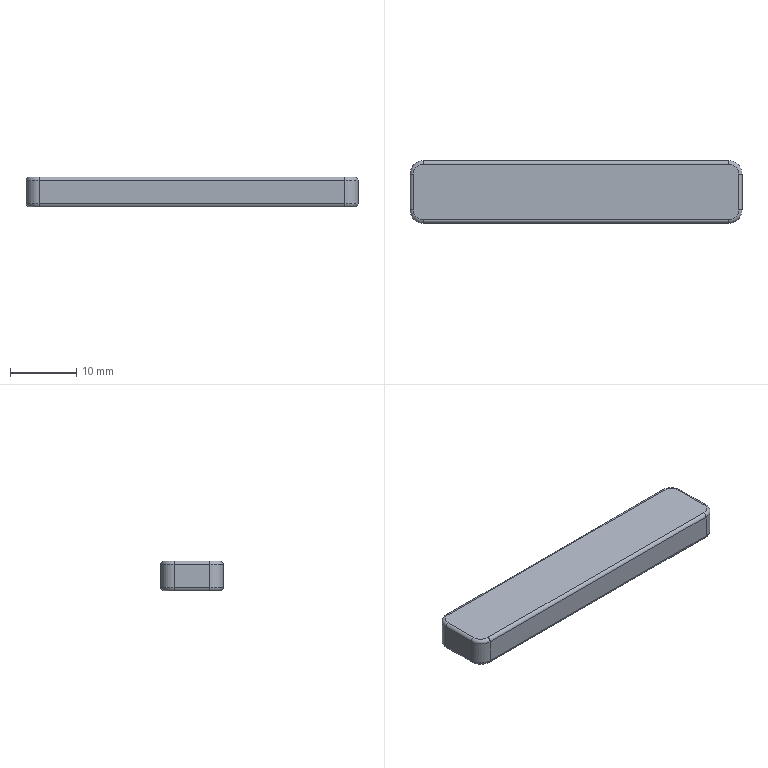Part | NX | features solid 2 | 1 solid | 26 faces | box 50 x 9.4 x 4.5 mm | volume 2087 mm3 | cylinder 12 | torus 8 | plane 6 | commonest cylinder face diameters 1 x8 4 x4
STEP:
#1=CARTESIAN_POINT('',(212.25,2183.3,2.5));
#2=VERTEX_POINT('',#1);
#3=CARTESIAN_POINT('',(214.25,2185.3,2.5));
#4=VERTEX_POINT('',#3);
#5=CARTESIAN_POINT('',(214.25,2183.3,2.5));
#6=DIRECTION('',(0.,0.,-1.));
#7=DIRECTION('',(-1.,0.,0.));
#8=AXIS2_PLACEMENT_3D('',#5,#6,#7);
#9=CIRCLE('',#8,2.);
#10=EDGE_CURVE('',#2,#4,#9,.T.);
#11=ORIENTED_EDGE('',*,*,#10,.F.);
#12=CARTESIAN_POINT('',(212.25,2183.3,6.));
#13=VERTEX_POINT('',#12);
#14=CARTESIAN_POINT('',(212.25,2183.3,2.5));
#15=DIRECTION('',(0.,0.,1.));
#16=VECTOR('',#15,1000.);
#17=LINE('',#14,#16);
#18=EDGE_CURVE('',#2,#13,#17,.T.);
#19=ORIENTED_EDGE('',*,*,#18,.T.);
#20=CARTESIAN_POINT('',(214.25,2185.3,6.));
#21=VERTEX_POINT('',#20);
#22=CARTESIAN_POINT('',(214.25,2183.3,6.));
#23=DIRECTION('',(0.,0.,1.));
#24=DIRECTION('',(0.,1.,0.));
#25=AXIS2_PLACEMENT_3D('',#22,#23,#24);
#26=CIRCLE('',#25,2.);
#27=EDGE_CURVE('',#21,#13,#26,.T.);
#28=ORIENTED_EDGE('',*,*,#27,.F.);
#29=CARTESIAN_POINT('',(214.25,2185.3,6.));
#30=DIRECTION('',(0.,0.,-1.));
#31=VECTOR('',#30,1000.);
#32=LINE('',#29,#31);
#33=EDGE_CURVE('',#21,#4,#32,.T.);
#34=ORIENTED_EDGE('',*,*,#33,.T.);
#35=EDGE_LOOP('',(#11,#19,#28,#34));
#36=FACE_BOUND('',#35,.T.);
#37=CARTESIAN_POINT('',(214.25,2183.3,4.25));
#38=DIRECTION('',(0.,0.,-1.));
#39=DIRECTION('',(1.,0.,0.));
#40=AXIS2_PLACEMENT_3D('',#37,#38,#39);
#41=CYLINDRICAL_SURFACE('',#40,2.);
#42=ADVANCED_FACE('',(#36),#41,.T.);
#43=CARTESIAN_POINT('',(260.25,2185.3,2.5));
#44=VERTEX_POINT('',#43);
#45=CARTESIAN_POINT('',(214.25,2185.3,2.5));
#46=DIRECTION('',(1.,0.,0.));
#47=VECTOR('',#46,1000.);
#48=LINE('',#45,#47);
#49=EDGE_CURVE('',#4,#44,#48,.T.);
#50=ORIENTED_EDGE('',*,*,#49,.F.);
#51=ORIENTED_EDGE('',*,*,#33,.F.);
#52=CARTESIAN_POINT('',(260.25,2185.3,6.));
#53=VERTEX_POINT('',#52);
#54=CARTESIAN_POINT('',(260.25,2185.3,6.));
#55=DIRECTION('',(-1.,0.,0.));
#56=VECTOR('',#55,1000.);
#57=LINE('',#54,#56);
#58=EDGE_CURVE('',#53,#21,#57,.T.);
#59=ORIENTED_EDGE('',*,*,#58,.F.);
#60=CARTESIAN_POINT('',(260.25,2185.3,2.5));
#61=DIRECTION('',(0.,0.,1.));
#62=VECTOR('',#61,1000.);
#63=LINE('',#60,#62);
#64=EDGE_CURVE('',#44,#53,#63,.T.);
#65=ORIENTED_EDGE('',*,*,#64,.F.);
#66=EDGE_LOOP('',(#50,#51,#59,#65));
#67=FACE_BOUND('',#66,.T.);
#68=CARTESIAN_POINT('',(264.862,2185.3,2.138));
#69=DIRECTION('',(0.,1.,0.));
#70=DIRECTION('',(0.,0.,-1.));
#71=AXIS2_PLACEMENT_3D('',#68,#69,#70);
#72=PLANE('',#71);
#73=ADVANCED_FACE('',(#67),#72,.T.);
#74=CARTESIAN_POINT('',(262.25,2183.3,2.5));
#75=VERTEX_POINT('',#74);
#76=CARTESIAN_POINT('',(260.25,2183.3,2.5));
#77=DIRECTION('',(0.,0.,-1.));
#78=DIRECTION('',(0.,1.,0.));
#79=AXIS2_PLACEMENT_3D('',#76,#77,#78);
#80=CIRCLE('',#79,2.);
#81=EDGE_CURVE('',#44,#75,#80,.T.);
#82=ORIENTED_EDGE('',*,*,#81,.F.);
#83=ORIENTED_EDGE('',*,*,#64,.T.);
#84=CARTESIAN_POINT('',(262.25,2183.3,6.));
#85=VERTEX_POINT('',#84);
#86=CARTESIAN_POINT('',(260.25,2183.3,6.));
#87=DIRECTION('',(0.,0.,1.));
#88=DIRECTION('',(1.,0.,0.));
#89=AXIS2_PLACEMENT_3D('',#86,#87,#88);
#90=CIRCLE('',#89,2.);
#91=EDGE_CURVE('',#85,#53,#90,.T.);
#92=ORIENTED_EDGE('',*,*,#91,.F.);
#93=CARTESIAN_POINT('',(262.25,2183.3,6.));
#94=DIRECTION('',(0.,0.,-1.));
#95=VECTOR('',#94,1000.);
#96=LINE('',#93,#95);
#97=EDGE_CURVE('',#85,#75,#96,.T.);
#98=ORIENTED_EDGE('',*,*,#97,.T.);
#99=EDGE_LOOP('',(#82,#83,#92,#98));
#100=FACE_BOUND('',#99,.T.);
#101=CARTESIAN_POINT('',(260.25,2183.3,4.25));
#102=DIRECTION('',(0.,0.,-1.));
#103=DIRECTION('',(1.,0.,0.));
#104=AXIS2_PLACEMENT_3D('',#101,#102,#103);
#105=CYLINDRICAL_SURFACE('',#104,2.);
#106=ADVANCED_FACE('',(#100),#105,.T.);
#107=CARTESIAN_POINT('',(262.25,2177.9,2.5));
#108=VERTEX_POINT('',#107);
#109=CARTESIAN_POINT('',(262.25,2183.3,2.5));
#110=DIRECTION('',(0.,-1.,0.));
#111=VECTOR('',#110,1000.);
#112=LINE('',#109,#111);
#113=EDGE_CURVE('',#75,#108,#112,.T.);
#114=ORIENTED_EDGE('',*,*,#113,.F.);
#115=ORIENTED_EDGE('',*,*,#97,.F.);
#116=CARTESIAN_POINT('',(262.25,2177.9,6.));
#117=VERTEX_POINT('',#116);
#118=CARTESIAN_POINT('',(262.25,2177.9,6.));
#119=DIRECTION('',(0.,1.,0.));
#120=VECTOR('',#119,1000.);
#121=LINE('',#118,#120);
#122=EDGE_CURVE('',#117,#85,#121,.T.);
#123=ORIENTED_EDGE('',*,*,#122,.F.);
#124=CARTESIAN_POINT('',(262.25,2177.9,2.5));
#125=DIRECTION('',(0.,0.,1.));
#126=VECTOR('',#125,1000.);
#127=LINE('',#124,#126);
#128=EDGE_CURVE('',#108,#117,#127,.T.);
#129=ORIENTED_EDGE('',*,*,#128,.F.);
#130=EDGE_LOOP('',(#114,#115,#123,#129));
#131=FACE_BOUND('',#130,.T.);
#132=CARTESIAN_POINT('',(262.25,2177.348,2.138));
#133=DIRECTION('',(1.,0.,0.));
#134=DIRECTION('',(0.,0.,1.));
#135=AXIS2_PLACEMENT_3D('',#132,#133,#134);
#136=PLANE('',#135);
#137=ADVANCED_FACE('',(#131),#136,.T.);
#138=CARTESIAN_POINT('',(260.25,2175.9,2.5));
#139=VERTEX_POINT('',#138);
#140=CARTESIAN_POINT('',(260.25,2177.9,2.5));
#141=DIRECTION('',(0.,0.,-1.));
#142=DIRECTION('',(1.,0.,0.));
#143=AXIS2_PLACEMENT_3D('',#140,#141,#142);
#144=CIRCLE('',#143,2.);
#145=EDGE_CURVE('',#108,#139,#144,.T.);
#146=ORIENTED_EDGE('',*,*,#145,.F.);
#147=ORIENTED_EDGE('',*,*,#128,.T.);
#148=CARTESIAN_POINT('',(260.25,2175.9,6.));
#149=VERTEX_POINT('',#148);
#150=CARTESIAN_POINT('',(260.25,2177.9,6.));
#151=DIRECTION('',(0.,0.,1.));
#152=DIRECTION('',(0.,-1.,0.));
#153=AXIS2_PLACEMENT_3D('',#150,#151,#152);
#154=CIRCLE('',#153,2.);
#155=EDGE_CURVE('',#149,#117,#154,.T.);
#156=ORIENTED_EDGE('',*,*,#155,.F.);
#157=CARTESIAN_POINT('',(260.25,2175.9,6.));
#158=DIRECTION('',(0.,0.,-1.));
#159=VECTOR('',#158,1000.);
#160=LINE('',#157,#159);
#161=EDGE_CURVE('',#149,#139,#160,.T.);
#162=ORIENTED_EDGE('',*,*,#161,.T.);
#163=EDGE_LOOP('',(#146,#147,#156,#162));
#164=FACE_BOUND('',#163,.T.);
#165=CARTESIAN_POINT('',(260.25,2177.9,4.25));
#166=DIRECTION('',(0.,0.,-1.));
#167=DIRECTION('',(1.,0.,0.));
#168=AXIS2_PLACEMENT_3D('',#165,#166,#167);
#169=CYLINDRICAL_SURFACE('',#168,2.);
#170=ADVANCED_FACE('',(#164),#169,.T.);
#171=CARTESIAN_POINT('',(214.25,2175.9,2.5));
#172=VERTEX_POINT('',#171);
#173=CARTESIAN_POINT('',(260.25,2175.9,2.5));
#174=DIRECTION('',(-1.,0.,0.));
#175=VECTOR('',#174,1000.);
#176=LINE('',#173,#175);
#177=EDGE_CURVE('',#139,#172,#176,.T.);
#178=ORIENTED_EDGE('',*,*,#177,.F.);
#179=ORIENTED_EDGE('',*,*,#161,.F.);
#180=CARTESIAN_POINT('',(214.25,2175.9,6.));
#181=VERTEX_POINT('',#180);
#182=CARTESIAN_POINT('',(214.25,2175.9,6.));
#183=DIRECTION('',(1.,0.,0.));
#184=VECTOR('',#183,1000.);
#185=LINE('',#182,#184);
#186=EDGE_CURVE('',#181,#149,#185,.T.);
#187=ORIENTED_EDGE('',*,*,#186,.F.);
#188=CARTESIAN_POINT('',(214.25,2175.9,2.5));
#189=DIRECTION('',(0.,0.,1.));
#190=VECTOR('',#189,1000.);
#191=LINE('',#188,#190);
#192=EDGE_CURVE('',#172,#181,#191,.T.);
#193=ORIENTED_EDGE('',*,*,#192,.F.);
#194=EDGE_LOOP('',(#178,#179,#187,#193));
#195=FACE_BOUND('',#194,.T.);
#196=CARTESIAN_POINT('',(209.638,2175.9,2.138));
#197=DIRECTION('',(0.,-1.,0.));
#198=DIRECTION('',(0.,0.,-1.));
#199=AXIS2_PLACEMENT_3D('',#196,#197,#198);
#200=PLANE('',#199);
#201=ADVANCED_FACE('',(#195),#200,.T.);
#202=CARTESIAN_POINT('',(212.25,2177.9,2.5));
#203=VERTEX_POINT('',#202);
#204=CARTESIAN_POINT('',(214.25,2177.9,2.5));
#205=DIRECTION('',(0.,0.,-1.));
#206=DIRECTION('',(0.,-1.,0.));
#207=AXIS2_PLACEMENT_3D('',#204,#205,#206);
#208=CIRCLE('',#207,2.);
#209=EDGE_CURVE('',#172,#203,#208,.T.);
#210=ORIENTED_EDGE('',*,*,#209,.F.);
#211=ORIENTED_EDGE('',*,*,#192,.T.);
#212=CARTESIAN_POINT('',(212.25,2177.9,6.));
#213=VERTEX_POINT('',#212);
#214=CARTESIAN_POINT('',(214.25,2177.9,6.));
#215=DIRECTION('',(0.,0.,1.));
#216=DIRECTION('',(-1.,0.,0.));
#217=AXIS2_PLACEMENT_3D('',#214,#215,#216);
#218=CIRCLE('',#217,2.);
#219=EDGE_CURVE('',#213,#181,#218,.T.);
#220=ORIENTED_EDGE('',*,*,#219,.F.);
#221=CARTESIAN_POINT('',(212.25,2177.9,6.));
#222=DIRECTION('',(0.,0.,-1.));
#223=VECTOR('',#222,1000.);
#224=LINE('',#221,#223);
#225=EDGE_CURVE('',#213,#203,#224,.T.);
#226=ORIENTED_EDGE('',*,*,#225,.T.);
#227=EDGE_LOOP('',(#210,#211,#220,#226));
#228=FACE_BOUND('',#227,.T.);
#229=CARTESIAN_POINT('',(214.25,2177.9,4.25));
#230=DIRECTION('',(0.,0.,-1.));
#231=DIRECTION('',(1.,0.,0.));
#232=AXIS2_PLACEMENT_3D('',#229,#230,#231);
#233=CYLINDRICAL_SURFACE('',#232,2.);
#234=ADVANCED_FACE('',(#228),#233,.T.);
#235=CARTESIAN_POINT('',(212.25,2177.9,2.5));
#236=DIRECTION('',(0.,1.,0.));
#237=VECTOR('',#236,1000.);
#238=LINE('',#235,#237);
#239=EDGE_CURVE('',#203,#2,#238,.T.);
#240=ORIENTED_EDGE('',*,*,#239,.F.);
#241=ORIENTED_EDGE('',*,*,#225,.F.);
#242=CARTESIAN_POINT('',(212.25,2183.3,6.));
#243=DIRECTION('',(0.,-1.,0.));
#244=VECTOR('',#243,1000.);
#245=LINE('',#242,#244);
#246=EDGE_CURVE('',#13,#213,#245,.T.);
#247=ORIENTED_EDGE('',*,*,#246,.F.);
#248=ORIENTED_EDGE('',*,*,#18,.F.);
#249=EDGE_LOOP('',(#240,#241,#247,#248));
#250=FACE_BOUND('',#249,.T.);
#251=CARTESIAN_POINT('',(212.25,2183.852,2.138));
#252=DIRECTION('',(-1.,0.,0.));
#253=DIRECTION('',(0.,0.,-1.));
#254=AXIS2_PLACEMENT_3D('',#251,#252,#253);
#255=PLANE('',#254);
#256=ADVANCED_FACE('',(#250),#255,.T.);
#257=ORIENTED_EDGE('',*,*,#246,.T.);
#258=CARTESIAN_POINT('',(212.75,2177.9,6.5));
#259=VERTEX_POINT('',#258);
#260=CARTESIAN_POINT('',(212.75,2177.9,6.));
#261=DIRECTION('',(0.,-1.,0.));
#262=DIRECTION('',(0.,0.,1.));
#263=AXIS2_PLACEMENT_3D('',#260,#261,#262);
#264=CIRCLE('',#263,0.5);
#265=EDGE_CURVE('',#259,#213,#264,.T.);
#266=ORIENTED_EDGE('',*,*,#265,.F.);
#267=CARTESIAN_POINT('',(212.75,2183.3,6.5));
#268=VERTEX_POINT('',#267);
#269=CARTESIAN_POINT('',(212.75,2177.9,6.5));
#270=DIRECTION('',(0.,1.,0.));
#271=VECTOR('',#270,1000.);
#272=LINE('',#269,#271);
#273=EDGE_CURVE('',#259,#268,#272,.T.);
#274=ORIENTED_EDGE('',*,*,#273,.T.);
#275=CARTESIAN_POINT('',(212.75,2183.3,6.));
#276=DIRECTION('',(0.,1.,0.));
#277=DIRECTION('',(-1.,0.,0.));
#278=AXIS2_PLACEMENT_3D('',#275,#276,#277);
#279=CIRCLE('',#278,0.5);
#280=EDGE_CURVE('',#13,#268,#279,.T.);
#281=ORIENTED_EDGE('',*,*,#280,.F.);
#282=EDGE_LOOP('',(#257,#266,#274,#281));
#283=FACE_BOUND('',#282,.T.);
#284=CARTESIAN_POINT('',(212.75,2180.6,6.));
#285=DIRECTION('',(0.,-1.,0.));
#286=DIRECTION('',(0.,0.,-1.));
#287=AXIS2_PLACEMENT_3D('',#284,#285,#286);
#288=CYLINDRICAL_SURFACE('',#287,0.5);
#289=ADVANCED_FACE('',(#283),#288,.T.);
#290=ORIENTED_EDGE('',*,*,#27,.T.);
#291=ORIENTED_EDGE('',*,*,#280,.T.);
#292=CARTESIAN_POINT('',(214.25,2184.8,6.5));
#293=VERTEX_POINT('',#292);
#294=CARTESIAN_POINT('',(214.25,2183.3,6.5));
#295=DIRECTION('',(0.,0.,1.));
#296=DIRECTION('',(0.,1.,0.));
#297=AXIS2_PLACEMENT_3D('',#294,#295,#296);
#298=CIRCLE('',#297,1.5);
#299=EDGE_CURVE('',#293,#268,#298,.T.);
#300=ORIENTED_EDGE('',*,*,#299,.F.);
#301=CARTESIAN_POINT('',(214.25,2184.8,6.));
#302=DIRECTION('',(-1.,0.,0.));
#303=DIRECTION('',(0.,0.,1.));
#304=AXIS2_PLACEMENT_3D('',#301,#302,#303);
#305=CIRCLE('',#304,0.5);
#306=EDGE_CURVE('',#293,#21,#305,.T.);
#307=ORIENTED_EDGE('',*,*,#306,.T.);
#308=EDGE_LOOP('',(#290,#291,#300,#307));
#309=FACE_BOUND('',#308,.T.);
#310=CARTESIAN_POINT('',(214.25,2183.3,6.));
#311=DIRECTION('',(0.,0.,1.));
#312=DIRECTION('',(0.,-1.,0.));
#313=AXIS2_PLACEMENT_3D('',#310,#311,#312);
#314=TOROIDAL_SURFACE('',#313,1.5,0.5);
#315=ADVANCED_FACE('',(#309),#314,.T.);
#316=ORIENTED_EDGE('',*,*,#58,.T.);
#317=ORIENTED_EDGE('',*,*,#306,.F.);
#318=CARTESIAN_POINT('',(260.25,2184.8,6.5));
#319=VERTEX_POINT('',#318);
#320=CARTESIAN_POINT('',(214.25,2184.8,6.5));
#321=DIRECTION('',(1.,0.,0.));
#322=VECTOR('',#321,1000.);
#323=LINE('',#320,#322);
#324=EDGE_CURVE('',#293,#319,#323,.T.);
#325=ORIENTED_EDGE('',*,*,#324,.T.);
#326=CARTESIAN_POINT('',(260.25,2184.8,6.));
#327=DIRECTION('',(1.,0.,0.));
#328=DIRECTION('',(0.,1.,0.));
#329=AXIS2_PLACEMENT_3D('',#326,#327,#328);
#330=CIRCLE('',#329,0.5);
#331=EDGE_CURVE('',#53,#319,#330,.T.);
#332=ORIENTED_EDGE('',*,*,#331,.F.);
#333=EDGE_LOOP('',(#316,#317,#325,#332));
#334=FACE_BOUND('',#333,.T.);
#335=CARTESIAN_POINT('',(237.25,2184.8,6.));
#336=DIRECTION('',(-1.,0.,0.));
#337=DIRECTION('',(0.,0.,-1.));
#338=AXIS2_PLACEMENT_3D('',#335,#336,#337);
#339=CYLINDRICAL_SURFACE('',#338,0.5);
#340=ADVANCED_FACE('',(#334),#339,.T.);
#341=ORIENTED_EDGE('',*,*,#91,.T.);
#342=ORIENTED_EDGE('',*,*,#331,.T.);
#343=CARTESIAN_POINT('',(261.75,2183.3,6.5));
#344=VERTEX_POINT('',#343);
#345=CARTESIAN_POINT('',(260.25,2183.3,6.5));
#346=DIRECTION('',(0.,0.,1.));
#347=DIRECTION('',(1.,0.,0.));
#348=AXIS2_PLACEMENT_3D('',#345,#346,#347);
#349=CIRCLE('',#348,1.5);
#350=EDGE_CURVE('',#344,#319,#349,.T.);
#351=ORIENTED_EDGE('',*,*,#350,.F.);
#352=CARTESIAN_POINT('',(261.75,2183.3,6.));
#353=DIRECTION('',(0.,1.,0.));
#354=DIRECTION('',(0.,0.,1.));
#355=AXIS2_PLACEMENT_3D('',#352,#353,#354);
#356=CIRCLE('',#355,0.5);
#357=EDGE_CURVE('',#344,#85,#356,.T.);
#358=ORIENTED_EDGE('',*,*,#357,.T.);
#359=EDGE_LOOP('',(#341,#342,#351,#358));
#360=FACE_BOUND('',#359,.T.);
#361=CARTESIAN_POINT('',(260.25,2183.3,6.));
#362=DIRECTION('',(0.,0.,1.));
#363=DIRECTION('',(-1.,0.,0.));
#364=AXIS2_PLACEMENT_3D('',#361,#362,#363);
#365=TOROIDAL_SURFACE('',#364,1.5,0.5);
#366=ADVANCED_FACE('',(#360),#365,.T.);
#367=ORIENTED_EDGE('',*,*,#122,.T.);
#368=ORIENTED_EDGE('',*,*,#357,.F.);
#369=CARTESIAN_POINT('',(261.75,2177.9,6.5));
#370=VERTEX_POINT('',#369);
#371=CARTESIAN_POINT('',(261.75,2183.3,6.5));
#372=DIRECTION('',(0.,-1.,0.));
#373=VECTOR('',#372,1000.);
#374=LINE('',#371,#373);
#375=EDGE_CURVE('',#344,#370,#374,.T.);
#376=ORIENTED_EDGE('',*,*,#375,.T.);
#377=CARTESIAN_POINT('',(261.75,2177.9,6.));
#378=DIRECTION('',(0.,-1.,0.));
#379=DIRECTION('',(1.,0.,0.));
#380=AXIS2_PLACEMENT_3D('',#377,#378,#379);
#381=CIRCLE('',#380,0.5);
#382=EDGE_CURVE('',#117,#370,#381,.T.);
#383=ORIENTED_EDGE('',*,*,#382,.F.);
#384=EDGE_LOOP('',(#367,#368,#376,#383));
#385=FACE_BOUND('',#384,.T.);
#386=CARTESIAN_POINT('',(261.75,2180.6,6.));
#387=DIRECTION('',(0.,1.,0.));
#388=DIRECTION('',(0.,0.,-1.));
#389=AXIS2_PLACEMENT_3D('',#386,#387,#388);
#390=CYLINDRICAL_SURFACE('',#389,0.5);
#391=ADVANCED_FACE('',(#385),#390,.T.);
#392=ORIENTED_EDGE('',*,*,#155,.T.);
#393=ORIENTED_EDGE('',*,*,#382,.T.);
#394=CARTESIAN_POINT('',(260.25,2176.4,6.5));
#395=VERTEX_POINT('',#394);
#396=CARTESIAN_POINT('',(260.25,2177.9,6.5));
#397=DIRECTION('',(0.,0.,1.));
#398=DIRECTION('',(0.,-1.,0.));
#399=AXIS2_PLACEMENT_3D('',#396,#397,#398);
#400=CIRCLE('',#399,1.5);
#401=EDGE_CURVE('',#395,#370,#400,.T.);
#402=ORIENTED_EDGE('',*,*,#401,.F.);
#403=CARTESIAN_POINT('',(260.25,2176.4,6.));
#404=DIRECTION('',(1.,0.,0.));
#405=DIRECTION('',(0.,0.,1.));
#406=AXIS2_PLACEMENT_3D('',#403,#404,#405);
#407=CIRCLE('',#406,0.5);
#408=EDGE_CURVE('',#395,#149,#407,.T.);
#409=ORIENTED_EDGE('',*,*,#408,.T.);
#410=EDGE_LOOP('',(#392,#393,#402,#409));
#411=FACE_BOUND('',#410,.T.);
#412=CARTESIAN_POINT('',(260.25,2177.9,6.));
#413=DIRECTION('',(0.,0.,1.));
#414=DIRECTION('',(-1.,0.,0.));
#415=AXIS2_PLACEMENT_3D('',#412,#413,#414);
#416=TOROIDAL_SURFACE('',#415,1.5,0.5);
#417=ADVANCED_FACE('',(#411),#416,.T.);
#418=ORIENTED_EDGE('',*,*,#186,.T.);
#419=ORIENTED_EDGE('',*,*,#408,.F.);
#420=CARTESIAN_POINT('',(214.25,2176.4,6.5));
#421=VERTEX_POINT('',#420);
#422=CARTESIAN_POINT('',(260.25,2176.4,6.5));
#423=DIRECTION('',(-1.,0.,0.));
#424=VECTOR('',#423,1000.);
#425=LINE('',#422,#424);
#426=EDGE_CURVE('',#395,#421,#425,.T.);
#427=ORIENTED_EDGE('',*,*,#426,.T.);
#428=CARTESIAN_POINT('',(214.25,2176.4,6.));
#429=DIRECTION('',(-1.,0.,0.));
#430=DIRECTION('',(0.,-1.,0.));
#431=AXIS2_PLACEMENT_3D('',#428,#429,#430);
#432=CIRCLE('',#431,0.5);
#433=EDGE_CURVE('',#181,#421,#432,.T.);
#434=ORIENTED_EDGE('',*,*,#433,.F.);
#435=EDGE_LOOP('',(#418,#419,#427,#434));
#436=FACE_BOUND('',#435,.T.);
#437=CARTESIAN_POINT('',(237.25,2176.4,6.));
#438=DIRECTION('',(1.,0.,0.));
#439=DIRECTION('',(0.,0.,1.));
#440=AXIS2_PLACEMENT_3D('',#437,#438,#439);
#441=CYLINDRICAL_SURFACE('',#440,0.5);
#442=ADVANCED_FACE('',(#436),#441,.T.);
#443=ORIENTED_EDGE('',*,*,#219,.T.);
#444=ORIENTED_EDGE('',*,*,#433,.T.);
#445=CARTESIAN_POINT('',(214.25,2177.9,6.5));
#446=DIRECTION('',(0.,0.,1.));
#447=DIRECTION('',(-1.,0.,0.));
#448=AXIS2_PLACEMENT_3D('',#445,#446,#447);
#449=CIRCLE('',#448,1.5);
#450=EDGE_CURVE('',#259,#421,#449,.T.);
#451=ORIENTED_EDGE('',*,*,#450,.F.);
#452=ORIENTED_EDGE('',*,*,#265,.T.);
#453=EDGE_LOOP('',(#443,#444,#451,#452));
#454=FACE_BOUND('',#453,.T.);
#455=CARTESIAN_POINT('',(214.25,2177.9,6.));
#456=DIRECTION('',(0.,0.,1.));
#457=DIRECTION('',(-1.,0.,0.));
#458=AXIS2_PLACEMENT_3D('',#455,#456,#457);
#459=TOROIDAL_SURFACE('',#458,1.5,0.5);
#460=ADVANCED_FACE('',(#454),#459,.T.);
#461=ORIENTED_EDGE('',*,*,#450,.T.);
#462=ORIENTED_EDGE('',*,*,#426,.F.);
#463=ORIENTED_EDGE('',*,*,#401,.T.);
#464=ORIENTED_EDGE('',*,*,#375,.F.);
#465=ORIENTED_EDGE('',*,*,#350,.T.);
#466=ORIENTED_EDGE('',*,*,#324,.F.);
#467=ORIENTED_EDGE('',*,*,#299,.T.);
#468=ORIENTED_EDGE('',*,*,#273,.F.);
#469=EDGE_LOOP('',(#461,#462,#463,#464,#465,#466,#467,#468));
#470=FACE_BOUND('',#469,.T.);
#471=CARTESIAN_POINT('',(207.838,2185.652,6.5));
#472=DIRECTION('',(0.,0.,1.));
#473=DIRECTION('',(-1.,0.,0.));
#474=AXIS2_PLACEMENT_3D('',#471,#472,#473);
#475=PLANE('',#474);
#476=ADVANCED_FACE('',(#470),#475,.T.);
#477=ORIENTED_EDGE('',*,*,#239,.T.);
#478=CARTESIAN_POINT('',(212.75,2183.3,2.));
#479=VERTEX_POINT('',#478);
#480=CARTESIAN_POINT('',(212.75,2183.3,2.5));
#481=DIRECTION('',(0.,1.,0.));
#482=DIRECTION('',(0.,0.,-1.));
#483=AXIS2_PLACEMENT_3D('',#480,#481,#482);
#484=CIRCLE('',#483,0.5);
#485=EDGE_CURVE('',#479,#2,#484,.T.);
#486=ORIENTED_EDGE('',*,*,#485,.F.);
#487=CARTESIAN_POINT('',(212.75,2177.9,2.));
#488=VERTEX_POINT('',#487);
#489=CARTESIAN_POINT('',(212.75,2183.3,2.));
#490=DIRECTION('',(0.,-1.,0.));
#491=VECTOR('',#490,1000.);
#492=LINE('',#489,#491);
#493=EDGE_CURVE('',#479,#488,#492,.T.);
#494=ORIENTED_EDGE('',*,*,#493,.T.);
#495=CARTESIAN_POINT('',(212.75,2177.9,2.5));
#496=DIRECTION('',(0.,-1.,0.));
#497=DIRECTION('',(-1.,0.,0.));
#498=AXIS2_PLACEMENT_3D('',#495,#496,#497);
#499=CIRCLE('',#498,0.5);
#500=EDGE_CURVE('',#203,#488,#499,.T.);
#501=ORIENTED_EDGE('',*,*,#500,.F.);
#502=EDGE_LOOP('',(#477,#486,#494,#501));
#503=FACE_BOUND('',#502,.T.);
#504=CARTESIAN_POINT('',(212.75,2180.6,2.5));
#505=DIRECTION('',(0.,1.,0.));
#506=DIRECTION('',(0.,0.,-1.));
#507=AXIS2_PLACEMENT_3D('',#504,#505,#506);
#508=CYLINDRICAL_SURFACE('',#507,0.5);
#509=ADVANCED_FACE('',(#503),#508,.T.);
#510=ORIENTED_EDGE('',*,*,#209,.T.);
#511=ORIENTED_EDGE('',*,*,#500,.T.);
#512=CARTESIAN_POINT('',(214.25,2176.4,2.));
#513=VERTEX_POINT('',#512);
#514=CARTESIAN_POINT('',(214.25,2177.9,2.));
#515=DIRECTION('',(0.,0.,-1.));
#516=DIRECTION('',(0.,-1.,0.));
#517=AXIS2_PLACEMENT_3D('',#514,#515,#516);
#518=CIRCLE('',#517,1.5);
#519=EDGE_CURVE('',#513,#488,#518,.T.);
#520=ORIENTED_EDGE('',*,*,#519,.F.);
#521=CARTESIAN_POINT('',(214.25,2176.4,2.5));
#522=DIRECTION('',(-1.,0.,0.));
#523=DIRECTION('',(0.,0.,-1.));
#524=AXIS2_PLACEMENT_3D('',#521,#522,#523);
#525=CIRCLE('',#524,0.5);
#526=EDGE_CURVE('',#513,#172,#525,.T.);
#527=ORIENTED_EDGE('',*,*,#526,.T.);
#528=EDGE_LOOP('',(#510,#511,#520,#527));
#529=FACE_BOUND('',#528,.T.);
#530=CARTESIAN_POINT('',(214.25,2177.9,2.5));
#531=DIRECTION('',(0.,0.,1.));
#532=DIRECTION('',(-1.,0.,0.));
#533=AXIS2_PLACEMENT_3D('',#530,#531,#532);
#534=TOROIDAL_SURFACE('',#533,1.5,0.5);
#535=ADVANCED_FACE('',(#529),#534,.T.);
#536=ORIENTED_EDGE('',*,*,#177,.T.);
#537=ORIENTED_EDGE('',*,*,#526,.F.);
#538=CARTESIAN_POINT('',(260.25,2176.4,2.));
#539=VERTEX_POINT('',#538);
#540=CARTESIAN_POINT('',(214.25,2176.4,2.));
#541=DIRECTION('',(1.,0.,0.));
#542=VECTOR('',#541,1000.);
#543=LINE('',#540,#542);
#544=EDGE_CURVE('',#513,#539,#543,.T.);
#545=ORIENTED_EDGE('',*,*,#544,.T.);
#546=CARTESIAN_POINT('',(260.25,2176.4,2.5));
#547=DIRECTION('',(1.,0.,0.));
#548=DIRECTION('',(0.,-1.,0.));
#549=AXIS2_PLACEMENT_3D('',#546,#547,#548);
#550=CIRCLE('',#549,0.5);
#551=EDGE_CURVE('',#139,#539,#550,.T.);
#552=ORIENTED_EDGE('',*,*,#551,.F.);
#553=EDGE_LOOP('',(#536,#537,#545,#552));
#554=FACE_BOUND('',#553,.T.);
#555=CARTESIAN_POINT('',(237.25,2176.4,2.5));
#556=DIRECTION('',(-1.,0.,0.));
#557=DIRECTION('',(0.,0.,-1.));
#558=AXIS2_PLACEMENT_3D('',#555,#556,#557);
#559=CYLINDRICAL_SURFACE('',#558,0.5);
#560=ADVANCED_FACE('',(#554),#559,.T.);
#561=ORIENTED_EDGE('',*,*,#145,.T.);
#562=ORIENTED_EDGE('',*,*,#551,.T.);
#563=CARTESIAN_POINT('',(261.75,2177.9,2.));
#564=VERTEX_POINT('',#563);
#565=CARTESIAN_POINT('',(260.25,2177.9,2.));
#566=DIRECTION('',(0.,0.,-1.));
#567=DIRECTION('',(1.,0.,0.));
#568=AXIS2_PLACEMENT_3D('',#565,#566,#567);
#569=CIRCLE('',#568,1.5);
#570=EDGE_CURVE('',#564,#539,#569,.T.);
#571=ORIENTED_EDGE('',*,*,#570,.F.);
#572=CARTESIAN_POINT('',(261.75,2177.9,2.5));
#573=DIRECTION('',(0.,-1.,0.));
#574=DIRECTION('',(0.,0.,-1.));
#575=AXIS2_PLACEMENT_3D('',#572,#573,#574);
#576=CIRCLE('',#575,0.5);
#577=EDGE_CURVE('',#564,#108,#576,.T.);
#578=ORIENTED_EDGE('',*,*,#577,.T.);
#579=EDGE_LOOP('',(#561,#562,#571,#578));
#580=FACE_BOUND('',#579,.T.);
#581=CARTESIAN_POINT('',(260.25,2177.9,2.5));
#582=DIRECTION('',(0.,0.,1.));
#583=DIRECTION('',(-1.,0.,0.));
#584=AXIS2_PLACEMENT_3D('',#581,#582,#583);
#585=TOROIDAL_SURFACE('',#584,1.5,0.5);
#586=ADVANCED_FACE('',(#580),#585,.T.);
#587=ORIENTED_EDGE('',*,*,#113,.T.);
#588=ORIENTED_EDGE('',*,*,#577,.F.);
#589=CARTESIAN_POINT('',(261.75,2183.3,2.));
#590=VERTEX_POINT('',#589);
#591=CARTESIAN_POINT('',(261.75,2177.9,2.));
#592=DIRECTION('',(0.,1.,0.));
#593=VECTOR('',#592,1000.);
#594=LINE('',#591,#593);
#595=EDGE_CURVE('',#564,#590,#594,.T.);
#596=ORIENTED_EDGE('',*,*,#595,.T.);
#597=CARTESIAN_POINT('',(261.75,2183.3,2.5));
#598=DIRECTION('',(0.,1.,0.));
#599=DIRECTION('',(1.,0.,0.));
#600=AXIS2_PLACEMENT_3D('',#597,#598,#599);
#601=CIRCLE('',#600,0.5);
#602=EDGE_CURVE('',#75,#590,#601,.T.);
#603=ORIENTED_EDGE('',*,*,#602,.F.);
#604=EDGE_LOOP('',(#587,#588,#596,#603));
#605=FACE_BOUND('',#604,.T.);
#606=CARTESIAN_POINT('',(261.75,2180.6,2.5));
#607=DIRECTION('',(0.,-1.,0.));
#608=DIRECTION('',(0.,0.,-1.));
#609=AXIS2_PLACEMENT_3D('',#606,#607,#608);
#610=CYLINDRICAL_SURFACE('',#609,0.5);
#611=ADVANCED_FACE('',(#605),#610,.T.);
#612=ORIENTED_EDGE('',*,*,#81,.T.);
#613=ORIENTED_EDGE('',*,*,#602,.T.);
#614=CARTESIAN_POINT('',(260.25,2184.8,2.));
#615=VERTEX_POINT('',#614);
#616=CARTESIAN_POINT('',(260.25,2183.3,2.));
#617=DIRECTION('',(0.,0.,-1.));
#618=DIRECTION('',(0.,1.,0.));
#619=AXIS2_PLACEMENT_3D('',#616,#617,#618);
#620=CIRCLE('',#619,1.5);
#621=EDGE_CURVE('',#615,#590,#620,.T.);
#622=ORIENTED_EDGE('',*,*,#621,.F.);
#623=CARTESIAN_POINT('',(260.25,2184.8,2.5));
#624=DIRECTION('',(1.,0.,0.));
#625=DIRECTION('',(0.,0.,-1.));
#626=AXIS2_PLACEMENT_3D('',#623,#624,#625);
#627=CIRCLE('',#626,0.5);
#628=EDGE_CURVE('',#615,#44,#627,.T.);
#629=ORIENTED_EDGE('',*,*,#628,.T.);
#630=EDGE_LOOP('',(#612,#613,#622,#629));
#631=FACE_BOUND('',#630,.T.);
#632=CARTESIAN_POINT('',(260.25,2183.3,2.5));
#633=DIRECTION('',(0.,0.,1.));
#634=DIRECTION('',(-1.,0.,0.));
#635=AXIS2_PLACEMENT_3D('',#632,#633,#634);
#636=TOROIDAL_SURFACE('',#635,1.5,0.5);
#637=ADVANCED_FACE('',(#631),#636,.T.);
#638=ORIENTED_EDGE('',*,*,#49,.T.);
#639=ORIENTED_EDGE('',*,*,#628,.F.);
#640=CARTESIAN_POINT('',(214.25,2184.8,2.));
#641=VERTEX_POINT('',#640);
#642=CARTESIAN_POINT('',(260.25,2184.8,2.));
#643=DIRECTION('',(-1.,0.,0.));
#644=VECTOR('',#643,1000.);
#645=LINE('',#642,#644);
#646=EDGE_CURVE('',#615,#641,#645,.T.);
#647=ORIENTED_EDGE('',*,*,#646,.T.);
#648=CARTESIAN_POINT('',(214.25,2184.8,2.5));
#649=DIRECTION('',(-1.,0.,0.));
#650=DIRECTION('',(0.,1.,0.));
#651=AXIS2_PLACEMENT_3D('',#648,#649,#650);
#652=CIRCLE('',#651,0.5);
#653=EDGE_CURVE('',#4,#641,#652,.T.);
#654=ORIENTED_EDGE('',*,*,#653,.F.);
#655=EDGE_LOOP('',(#638,#639,#647,#654));
#656=FACE_BOUND('',#655,.T.);
#657=CARTESIAN_POINT('',(237.25,2184.8,2.5));
#658=DIRECTION('',(1.,0.,0.));
#659=DIRECTION('',(0.,0.,1.));
#660=AXIS2_PLACEMENT_3D('',#657,#658,#659);
#661=CYLINDRICAL_SURFACE('',#660,0.5);
#662=ADVANCED_FACE('',(#656),#661,.T.);
#663=ORIENTED_EDGE('',*,*,#10,.T.);
#664=ORIENTED_EDGE('',*,*,#653,.T.);
#665=CARTESIAN_POINT('',(214.25,2183.3,2.));
#666=DIRECTION('',(0.,0.,-1.));
#667=DIRECTION('',(-1.,0.,0.));
#668=AXIS2_PLACEMENT_3D('',#665,#666,#667);
#669=CIRCLE('',#668,1.5);
#670=EDGE_CURVE('',#479,#641,#669,.T.);
#671=ORIENTED_EDGE('',*,*,#670,.F.);
#672=ORIENTED_EDGE('',*,*,#485,.T.);
#673=EDGE_LOOP('',(#663,#664,#671,#672));
#674=FACE_BOUND('',#673,.T.);
#675=CARTESIAN_POINT('',(214.25,2183.3,2.5));
#676=DIRECTION('',(0.,0.,1.));
#677=DIRECTION('',(-1.,0.,0.));
#678=AXIS2_PLACEMENT_3D('',#675,#676,#677);
#679=TOROIDAL_SURFACE('',#678,1.5,0.5);
#680=ADVANCED_FACE('',(#674),#679,.T.);
#681=ORIENTED_EDGE('',*,*,#544,.F.);
#682=ORIENTED_EDGE('',*,*,#519,.T.);
#683=ORIENTED_EDGE('',*,*,#493,.F.);
#684=ORIENTED_EDGE('',*,*,#670,.T.);
#685=ORIENTED_EDGE('',*,*,#646,.F.);
#686=ORIENTED_EDGE('',*,*,#621,.T.);
#687=ORIENTED_EDGE('',*,*,#595,.F.);
#688=ORIENTED_EDGE('',*,*,#570,.T.);
#689=EDGE_LOOP('',(#681,#682,#683,#684,#685,#686,#687,#688));
#690=FACE_BOUND('',#689,.T.);
#691=CARTESIAN_POINT('',(207.838,2185.652,2.));
#692=DIRECTION('',(0.,0.,-1.));
#693=DIRECTION('',(1.,0.,0.));
#694=AXIS2_PLACEMENT_3D('',#691,#692,#693);
#695=PLANE('',#694);
#696=ADVANCED_FACE('',(#690),#695,.T.);
#697=CLOSED_SHELL('',(#42,#73,#106,#137,#170,#201,#234,#256,#289,#315,#340,#366,#391,#417,#442,#460,#476,#509,#535,#560,#586,#611,#637,#662,#680,#696));
#698=MANIFOLD_SOLID_BREP('',#697);
#699=(LENGTH_UNIT()NAMED_UNIT(*)SI_UNIT(.MILLI.,.METRE.));
#700=UNCERTAINTY_MEASURE_WITH_UNIT(LENGTH_MEASURE(0.00001),#699,'','');
#701=(NAMED_UNIT(*)PLANE_ANGLE_UNIT()SI_UNIT($,.RADIAN.));
#702=(NAMED_UNIT(*)SI_UNIT($,.STERADIAN.)SOLID_ANGLE_UNIT());
#703=(GEOMETRIC_REPRESENTATION_CONTEXT(3)GLOBAL_UNCERTAINTY_ASSIGNED_CONTEXT((#700))GLOBAL_UNIT_ASSIGNED_CONTEXT((#699,#701,#702))REPRESENTATION_CONTEXT('',''));
#704=ADVANCED_BREP_SHAPE_REPRESENTATION('',(#698),#703);